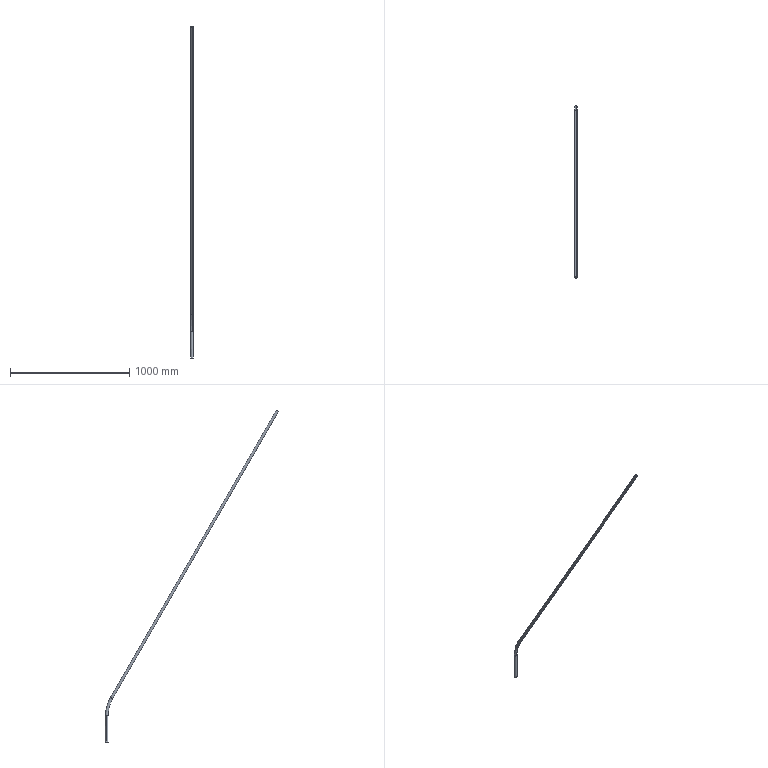Part | SolidWorks | features Sweep 1 | 1 solid | 14 faces | box 22 x 1453 x 2786 mm | volume 397136 mm3 | cylinder 8 | torus 4 | plane 2 | commonest cylinder face diameters 18 x4 22 x4
STEP:
#1=CARTESIAN_POINT('',(-9.,0.,219.615));
#2=VERTEX_POINT('',#1);
#3=CARTESIAN_POINT('',(0.,9.,219.615));
#4=VERTEX_POINT('',#3);
#5=CARTESIAN_POINT('',(0.,0.,219.615));
#6=DIRECTION('',(0.,0.,-1.));
#7=DIRECTION('',(1.,0.,0.));
#8=AXIS2_PLACEMENT_3D('',#5,#6,#7);
#9=CIRCLE('',#8,9.);
#10=EDGE_CURVE('',#2,#4,#9,.T.);
#11=ORIENTED_EDGE('',*,*,#10,.T.);
#12=CARTESIAN_POINT('',(0.,-32.398,374.115));
#13=VERTEX_POINT('',#12);
#14=CARTESIAN_POINT('',(0.,-300.,219.615));
#15=DIRECTION('',(1.,0.,0.));
#16=DIRECTION('',(0.,0.,-1.));
#17=AXIS2_PLACEMENT_3D('',#14,#15,#16);
#18=CIRCLE('',#17,309.);
#19=EDGE_CURVE('',#4,#13,#18,.T.);
#20=ORIENTED_EDGE('',*,*,#19,.T.);
#21=CARTESIAN_POINT('',(0.,-47.987,365.115));
#22=VERTEX_POINT('',#21);
#23=CARTESIAN_POINT('',(0.,-40.192,369.615));
#24=DIRECTION('',(0.,0.5,-0.866));
#25=DIRECTION('',(1.,0.,0.));
#26=AXIS2_PLACEMENT_3D('',#23,#24,#25);
#27=CIRCLE('',#26,9.);
#28=EDGE_CURVE('',#22,#13,#27,.T.);
#29=ORIENTED_EDGE('',*,*,#28,.F.);
#30=CARTESIAN_POINT('',(0.,-9.,219.615));
#31=VERTEX_POINT('',#30);
#32=CARTESIAN_POINT('',(0.,-300.,219.615));
#33=DIRECTION('',(1.,0.,0.));
#34=DIRECTION('',(0.,0.,-1.));
#35=AXIS2_PLACEMENT_3D('',#32,#33,#34);
#36=CIRCLE('',#35,291.);
#37=EDGE_CURVE('',#31,#22,#36,.T.);
#38=ORIENTED_EDGE('',*,*,#37,.F.);
#39=CARTESIAN_POINT('',(0.,0.,219.615));
#40=DIRECTION('',(0.,0.,-1.));
#41=DIRECTION('',(1.,0.,0.));
#42=AXIS2_PLACEMENT_3D('',#39,#40,#41);
#43=CIRCLE('',#42,9.);
#44=EDGE_CURVE('',#31,#2,#43,.T.);
#45=ORIENTED_EDGE('',*,*,#44,.T.);
#46=EDGE_LOOP('',(#11,#20,#29,#38,#45));
#47=FACE_OUTER_BOUND('',#46,.T.);
#48=CARTESIAN_POINT('',(0.,-300.,219.615));
#49=DIRECTION('',(1.,0.,0.));
#50=DIRECTION('',(0.,0.,-1.));
#51=AXIS2_PLACEMENT_3D('',#48,#49,#50);
#52=TOROIDAL_SURFACE('',#51,300.,9.);
#53=ADVANCED_FACE('',(#47),#52,.F.);
#54=CARTESIAN_POINT('',(11.,0.,219.615));
#55=VERTEX_POINT('',#54);
#56=CARTESIAN_POINT('',(0.,11.,219.615));
#57=VERTEX_POINT('',#56);
#58=CARTESIAN_POINT('',(0.,0.,219.615));
#59=DIRECTION('',(0.,0.,1.));
#60=DIRECTION('',(1.,0.,0.));
#61=AXIS2_PLACEMENT_3D('',#58,#59,#60);
#62=CIRCLE('',#61,11.);
#63=EDGE_CURVE('',#55,#57,#62,.T.);
#64=ORIENTED_EDGE('',*,*,#63,.T.);
#65=CARTESIAN_POINT('',(0.,-30.666,375.115));
#66=VERTEX_POINT('',#65);
#67=CARTESIAN_POINT('',(0.,-300.,219.615));
#68=DIRECTION('',(1.,0.,0.));
#69=DIRECTION('',(0.,0.,-1.));
#70=AXIS2_PLACEMENT_3D('',#67,#68,#69);
#71=CIRCLE('',#70,311.);
#72=EDGE_CURVE('',#57,#66,#71,.T.);
#73=ORIENTED_EDGE('',*,*,#72,.T.);
#74=CARTESIAN_POINT('',(0.,-49.719,364.115));
#75=VERTEX_POINT('',#74);
#76=CARTESIAN_POINT('',(0.,-40.192,369.615));
#77=DIRECTION('',(0.,-0.5,0.866));
#78=DIRECTION('',(1.,0.,0.));
#79=AXIS2_PLACEMENT_3D('',#76,#77,#78);
#80=CIRCLE('',#79,11.);
#81=EDGE_CURVE('',#75,#66,#80,.T.);
#82=ORIENTED_EDGE('',*,*,#81,.F.);
#83=CARTESIAN_POINT('',(0.,-11.,219.615));
#84=VERTEX_POINT('',#83);
#85=CARTESIAN_POINT('',(0.,-300.,219.615));
#86=DIRECTION('',(1.,0.,0.));
#87=DIRECTION('',(0.,0.,-1.));
#88=AXIS2_PLACEMENT_3D('',#85,#86,#87);
#89=CIRCLE('',#88,289.);
#90=EDGE_CURVE('',#84,#75,#89,.T.);
#91=ORIENTED_EDGE('',*,*,#90,.F.);
#92=CARTESIAN_POINT('',(0.,0.,219.615));
#93=DIRECTION('',(0.,0.,1.));
#94=DIRECTION('',(1.,0.,0.));
#95=AXIS2_PLACEMENT_3D('',#92,#93,#94);
#96=CIRCLE('',#95,11.);
#97=EDGE_CURVE('',#84,#55,#96,.T.);
#98=ORIENTED_EDGE('',*,*,#97,.T.);
#99=EDGE_LOOP('',(#64,#73,#82,#91,#98));
#100=FACE_OUTER_BOUND('',#99,.T.);
#101=CARTESIAN_POINT('',(0.,-300.,219.615));
#102=DIRECTION('',(1.,0.,0.));
#103=DIRECTION('',(0.,0.,-1.));
#104=AXIS2_PLACEMENT_3D('',#101,#102,#103);
#105=TOROIDAL_SURFACE('',#104,300.,11.);
#106=ADVANCED_FACE('',(#100),#105,.T.);
#107=ORIENTED_EDGE('',*,*,#28,.T.);
#108=CARTESIAN_POINT('',(0.,-1424.206,2784.797));
#109=VERTEX_POINT('',#108);
#110=CARTESIAN_POINT('',(0.,-32.398,374.115));
#111=DIRECTION('',(0.,-0.5,0.866));
#112=VECTOR('',#111,1000.);
#113=LINE('',#110,#112);
#114=EDGE_CURVE('',#13,#109,#113,.T.);
#115=ORIENTED_EDGE('',*,*,#114,.T.);
#116=CARTESIAN_POINT('',(0.,-1439.794,2775.797));
#117=VERTEX_POINT('',#116);
#118=CARTESIAN_POINT('',(0.,-1432.,2780.297));
#119=DIRECTION('',(0.,0.5,-0.866));
#120=DIRECTION('',(1.,0.,0.));
#121=AXIS2_PLACEMENT_3D('',#118,#119,#120);
#122=CIRCLE('',#121,9.);
#123=EDGE_CURVE('',#117,#109,#122,.T.);
#124=ORIENTED_EDGE('',*,*,#123,.F.);
#125=CARTESIAN_POINT('',(0.,-47.987,365.115));
#126=DIRECTION('',(0.,-0.5,0.866));
#127=VECTOR('',#126,1000.);
#128=LINE('',#125,#127);
#129=EDGE_CURVE('',#22,#117,#128,.T.);
#130=ORIENTED_EDGE('',*,*,#129,.F.);
#131=EDGE_LOOP('',(#107,#115,#124,#130));
#132=FACE_OUTER_BOUND('',#131,.T.);
#133=CARTESIAN_POINT('',(0.,-40.192,369.615));
#134=DIRECTION('',(0.,-0.5,0.866));
#135=DIRECTION('',(0.,-0.866,-0.5));
#136=AXIS2_PLACEMENT_3D('',#133,#134,#135);
#137=CYLINDRICAL_SURFACE('',#136,9.);
#138=ADVANCED_FACE('',(#132),#137,.F.);
#139=CARTESIAN_POINT('',(9.,0.,0.));
#140=VERTEX_POINT('',#139);
#141=CARTESIAN_POINT('',(-9.,0.,0.));
#142=VERTEX_POINT('',#141);
#143=CARTESIAN_POINT('',(0.,0.,0.));
#144=DIRECTION('',(0.,0.,-1.));
#145=DIRECTION('',(1.,0.,0.));
#146=AXIS2_PLACEMENT_3D('',#143,#144,#145);
#147=CIRCLE('',#146,9.);
#148=EDGE_CURVE('',#140,#142,#147,.T.);
#149=ORIENTED_EDGE('',*,*,#148,.T.);
#150=CARTESIAN_POINT('',(-9.,0.,0.));
#151=DIRECTION('',(0.,0.,1.));
#152=VECTOR('',#151,1000.);
#153=LINE('',#150,#152);
#154=EDGE_CURVE('',#142,#2,#153,.T.);
#155=ORIENTED_EDGE('',*,*,#154,.T.);
#156=ORIENTED_EDGE('',*,*,#44,.F.);
#157=CARTESIAN_POINT('',(9.,0.,219.615));
#158=VERTEX_POINT('',#157);
#159=CARTESIAN_POINT('',(0.,0.,219.615));
#160=DIRECTION('',(0.,0.,-1.));
#161=DIRECTION('',(1.,0.,0.));
#162=AXIS2_PLACEMENT_3D('',#159,#160,#161);
#163=CIRCLE('',#162,9.);
#164=EDGE_CURVE('',#158,#31,#163,.T.);
#165=ORIENTED_EDGE('',*,*,#164,.F.);
#166=CARTESIAN_POINT('',(9.,0.,0.));
#167=DIRECTION('',(0.,0.,1.));
#168=VECTOR('',#167,1000.);
#169=LINE('',#166,#168);
#170=EDGE_CURVE('',#140,#158,#169,.T.);
#171=ORIENTED_EDGE('',*,*,#170,.F.);
#172=EDGE_LOOP('',(#149,#155,#156,#165,#171));
#173=FACE_OUTER_BOUND('',#172,.T.);
#174=CARTESIAN_POINT('',(0.,0.,0.));
#175=DIRECTION('',(0.,0.,1.));
#176=DIRECTION('',(1.,0.,0.));
#177=AXIS2_PLACEMENT_3D('',#174,#175,#176);
#178=CYLINDRICAL_SURFACE('',#177,9.);
#179=ADVANCED_FACE('',(#173),#178,.F.);
#180=ORIENTED_EDGE('',*,*,#81,.T.);
#181=CARTESIAN_POINT('',(0.,-1422.474,2785.797));
#182=VERTEX_POINT('',#181);
#183=CARTESIAN_POINT('',(0.,-30.666,375.115));
#184=DIRECTION('',(0.,-0.5,0.866));
#185=VECTOR('',#184,1000.);
#186=LINE('',#183,#185);
#187=EDGE_CURVE('',#66,#182,#186,.T.);
#188=ORIENTED_EDGE('',*,*,#187,.T.);
#189=CARTESIAN_POINT('',(0.,-1441.526,2774.797));
#190=VERTEX_POINT('',#189);
#191=CARTESIAN_POINT('',(0.,-1432.,2780.297));
#192=DIRECTION('',(0.,-0.5,0.866));
#193=DIRECTION('',(1.,0.,0.));
#194=AXIS2_PLACEMENT_3D('',#191,#192,#193);
#195=CIRCLE('',#194,11.);
#196=EDGE_CURVE('',#190,#182,#195,.T.);
#197=ORIENTED_EDGE('',*,*,#196,.F.);
#198=CARTESIAN_POINT('',(0.,-49.719,364.115));
#199=DIRECTION('',(0.,-0.5,0.866));
#200=VECTOR('',#199,1000.);
#201=LINE('',#198,#200);
#202=EDGE_CURVE('',#75,#190,#201,.T.);
#203=ORIENTED_EDGE('',*,*,#202,.F.);
#204=EDGE_LOOP('',(#180,#188,#197,#203));
#205=FACE_OUTER_BOUND('',#204,.T.);
#206=CARTESIAN_POINT('',(0.,-40.192,369.615));
#207=DIRECTION('',(0.,-0.5,0.866));
#208=DIRECTION('',(0.,-0.866,-0.5));
#209=AXIS2_PLACEMENT_3D('',#206,#207,#208);
#210=CYLINDRICAL_SURFACE('',#209,11.);
#211=ADVANCED_FACE('',(#205),#210,.T.);
#212=CARTESIAN_POINT('',(11.,0.,0.));
#213=VERTEX_POINT('',#212);
#214=CARTESIAN_POINT('',(-11.,0.,0.));
#215=VERTEX_POINT('',#214);
#216=CARTESIAN_POINT('',(0.,0.,0.));
#217=DIRECTION('',(0.,0.,1.));
#218=DIRECTION('',(1.,0.,0.));
#219=AXIS2_PLACEMENT_3D('',#216,#217,#218);
#220=CIRCLE('',#219,11.);
#221=EDGE_CURVE('',#213,#215,#220,.T.);
#222=ORIENTED_EDGE('',*,*,#221,.T.);
#223=CARTESIAN_POINT('',(-11.,0.,219.615));
#224=VERTEX_POINT('',#223);
#225=CARTESIAN_POINT('',(-11.,0.,0.));
#226=DIRECTION('',(0.,0.,1.));
#227=VECTOR('',#226,1000.);
#228=LINE('',#225,#227);
#229=EDGE_CURVE('',#215,#224,#228,.T.);
#230=ORIENTED_EDGE('',*,*,#229,.T.);
#231=CARTESIAN_POINT('',(0.,0.,219.615));
#232=DIRECTION('',(0.,0.,1.));
#233=DIRECTION('',(1.,0.,0.));
#234=AXIS2_PLACEMENT_3D('',#231,#232,#233);
#235=CIRCLE('',#234,11.);
#236=EDGE_CURVE('',#57,#224,#235,.T.);
#237=ORIENTED_EDGE('',*,*,#236,.F.);
#238=ORIENTED_EDGE('',*,*,#63,.F.);
#239=CARTESIAN_POINT('',(11.,0.,0.));
#240=DIRECTION('',(0.,0.,1.));
#241=VECTOR('',#240,1000.);
#242=LINE('',#239,#241);
#243=EDGE_CURVE('',#213,#55,#242,.T.);
#244=ORIENTED_EDGE('',*,*,#243,.F.);
#245=EDGE_LOOP('',(#222,#230,#237,#238,#244));
#246=FACE_OUTER_BOUND('',#245,.T.);
#247=CARTESIAN_POINT('',(0.,0.,0.));
#248=DIRECTION('',(0.,0.,1.));
#249=DIRECTION('',(1.,0.,0.));
#250=AXIS2_PLACEMENT_3D('',#247,#248,#249);
#251=CYLINDRICAL_SURFACE('',#250,11.);
#252=ADVANCED_FACE('',(#246),#251,.T.);
#253=ORIENTED_EDGE('',*,*,#114,.F.);
#254=CARTESIAN_POINT('',(0.,-40.192,369.615));
#255=DIRECTION('',(0.,0.5,-0.866));
#256=DIRECTION('',(1.,0.,0.));
#257=AXIS2_PLACEMENT_3D('',#254,#255,#256);
#258=CIRCLE('',#257,9.);
#259=EDGE_CURVE('',#13,#22,#258,.T.);
#260=ORIENTED_EDGE('',*,*,#259,.T.);
#261=ORIENTED_EDGE('',*,*,#129,.T.);
#262=CARTESIAN_POINT('',(0.,-1432.,2780.297));
#263=DIRECTION('',(0.,0.5,-0.866));
#264=DIRECTION('',(1.,0.,0.));
#265=AXIS2_PLACEMENT_3D('',#262,#263,#264);
#266=CIRCLE('',#265,9.);
#267=EDGE_CURVE('',#109,#117,#266,.T.);
#268=ORIENTED_EDGE('',*,*,#267,.F.);
#269=EDGE_LOOP('',(#253,#260,#261,#268));
#270=FACE_OUTER_BOUND('',#269,.T.);
#271=CARTESIAN_POINT('',(0.,-40.192,369.615));
#272=DIRECTION('',(0.,-0.5,0.866));
#273=DIRECTION('',(0.,-0.866,-0.5));
#274=AXIS2_PLACEMENT_3D('',#271,#272,#273);
#275=CYLINDRICAL_SURFACE('',#274,9.);
#276=ADVANCED_FACE('',(#270),#275,.F.);
#277=ORIENTED_EDGE('',*,*,#19,.F.);
#278=CARTESIAN_POINT('',(0.,0.,219.615));
#279=DIRECTION('',(0.,0.,-1.));
#280=DIRECTION('',(1.,0.,0.));
#281=AXIS2_PLACEMENT_3D('',#278,#279,#280);
#282=CIRCLE('',#281,9.);
#283=EDGE_CURVE('',#4,#158,#282,.T.);
#284=ORIENTED_EDGE('',*,*,#283,.T.);
#285=ORIENTED_EDGE('',*,*,#164,.T.);
#286=ORIENTED_EDGE('',*,*,#37,.T.);
#287=ORIENTED_EDGE('',*,*,#259,.F.);
#288=EDGE_LOOP('',(#277,#284,#285,#286,#287));
#289=FACE_OUTER_BOUND('',#288,.T.);
#290=CARTESIAN_POINT('',(0.,-300.,219.615));
#291=DIRECTION('',(1.,0.,0.));
#292=DIRECTION('',(0.,0.,-1.));
#293=AXIS2_PLACEMENT_3D('',#290,#291,#292);
#294=TOROIDAL_SURFACE('',#293,300.,9.);
#295=ADVANCED_FACE('',(#289),#294,.F.);
#296=ORIENTED_EDGE('',*,*,#154,.F.);
#297=CARTESIAN_POINT('',(0.,0.,0.));
#298=DIRECTION('',(0.,0.,-1.));
#299=DIRECTION('',(1.,0.,0.));
#300=AXIS2_PLACEMENT_3D('',#297,#298,#299);
#301=CIRCLE('',#300,9.);
#302=EDGE_CURVE('',#142,#140,#301,.T.);
#303=ORIENTED_EDGE('',*,*,#302,.T.);
#304=ORIENTED_EDGE('',*,*,#170,.T.);
#305=ORIENTED_EDGE('',*,*,#283,.F.);
#306=ORIENTED_EDGE('',*,*,#10,.F.);
#307=EDGE_LOOP('',(#296,#303,#304,#305,#306));
#308=FACE_OUTER_BOUND('',#307,.T.);
#309=CARTESIAN_POINT('',(0.,0.,0.));
#310=DIRECTION('',(0.,0.,1.));
#311=DIRECTION('',(1.,0.,0.));
#312=AXIS2_PLACEMENT_3D('',#309,#310,#311);
#313=CYLINDRICAL_SURFACE('',#312,9.);
#314=ADVANCED_FACE('',(#308),#313,.F.);
#315=ORIENTED_EDGE('',*,*,#123,.T.);
#316=ORIENTED_EDGE('',*,*,#267,.T.);
#317=EDGE_LOOP('',(#315,#316));
#318=FACE_BOUND('',#317,.T.);
#319=ORIENTED_EDGE('',*,*,#196,.T.);
#320=CARTESIAN_POINT('',(0.,-1432.,2780.297));
#321=DIRECTION('',(0.,-0.5,0.866));
#322=DIRECTION('',(1.,0.,0.));
#323=AXIS2_PLACEMENT_3D('',#320,#321,#322);
#324=CIRCLE('',#323,11.);
#325=EDGE_CURVE('',#182,#190,#324,.T.);
#326=ORIENTED_EDGE('',*,*,#325,.T.);
#327=EDGE_LOOP('',(#319,#326));
#328=FACE_OUTER_BOUND('',#327,.T.);
#329=CARTESIAN_POINT('',(0.,-1432.,2780.297));
#330=DIRECTION('',(0.,-0.5,0.866));
#331=DIRECTION('',(1.,0.,0.));
#332=AXIS2_PLACEMENT_3D('',#329,#330,#331);
#333=PLANE('',#332);
#334=ADVANCED_FACE('',(#318,#328),#333,.T.);
#335=ORIENTED_EDGE('',*,*,#148,.F.);
#336=ORIENTED_EDGE('',*,*,#302,.F.);
#337=EDGE_LOOP('',(#335,#336));
#338=FACE_BOUND('',#337,.T.);
#339=ORIENTED_EDGE('',*,*,#221,.F.);
#340=CARTESIAN_POINT('',(0.,0.,0.));
#341=DIRECTION('',(0.,0.,1.));
#342=DIRECTION('',(1.,0.,0.));
#343=AXIS2_PLACEMENT_3D('',#340,#341,#342);
#344=CIRCLE('',#343,11.);
#345=EDGE_CURVE('',#215,#213,#344,.T.);
#346=ORIENTED_EDGE('',*,*,#345,.F.);
#347=EDGE_LOOP('',(#339,#346));
#348=FACE_OUTER_BOUND('',#347,.T.);
#349=CARTESIAN_POINT('',(0.,0.,0.));
#350=DIRECTION('',(0.,0.,1.));
#351=DIRECTION('',(1.,0.,0.));
#352=AXIS2_PLACEMENT_3D('',#349,#350,#351);
#353=PLANE('',#352);
#354=ADVANCED_FACE('',(#338,#348),#353,.F.);
#355=ORIENTED_EDGE('',*,*,#187,.F.);
#356=CARTESIAN_POINT('',(0.,-40.192,369.615));
#357=DIRECTION('',(0.,-0.5,0.866));
#358=DIRECTION('',(1.,0.,0.));
#359=AXIS2_PLACEMENT_3D('',#356,#357,#358);
#360=CIRCLE('',#359,11.);
#361=EDGE_CURVE('',#66,#75,#360,.T.);
#362=ORIENTED_EDGE('',*,*,#361,.T.);
#363=ORIENTED_EDGE('',*,*,#202,.T.);
#364=ORIENTED_EDGE('',*,*,#325,.F.);
#365=EDGE_LOOP('',(#355,#362,#363,#364));
#366=FACE_OUTER_BOUND('',#365,.T.);
#367=CARTESIAN_POINT('',(0.,-40.192,369.615));
#368=DIRECTION('',(0.,-0.5,0.866));
#369=DIRECTION('',(0.,-0.866,-0.5));
#370=AXIS2_PLACEMENT_3D('',#367,#368,#369);
#371=CYLINDRICAL_SURFACE('',#370,11.);
#372=ADVANCED_FACE('',(#366),#371,.T.);
#373=ORIENTED_EDGE('',*,*,#72,.F.);
#374=ORIENTED_EDGE('',*,*,#236,.T.);
#375=CARTESIAN_POINT('',(0.,0.,219.615));
#376=DIRECTION('',(0.,0.,1.));
#377=DIRECTION('',(1.,0.,0.));
#378=AXIS2_PLACEMENT_3D('',#375,#376,#377);
#379=CIRCLE('',#378,11.);
#380=EDGE_CURVE('',#224,#84,#379,.T.);
#381=ORIENTED_EDGE('',*,*,#380,.T.);
#382=ORIENTED_EDGE('',*,*,#90,.T.);
#383=ORIENTED_EDGE('',*,*,#361,.F.);
#384=EDGE_LOOP('',(#373,#374,#381,#382,#383));
#385=FACE_OUTER_BOUND('',#384,.T.);
#386=CARTESIAN_POINT('',(0.,-300.,219.615));
#387=DIRECTION('',(1.,0.,0.));
#388=DIRECTION('',(0.,0.,-1.));
#389=AXIS2_PLACEMENT_3D('',#386,#387,#388);
#390=TOROIDAL_SURFACE('',#389,300.,11.);
#391=ADVANCED_FACE('',(#385),#390,.T.);
#392=ORIENTED_EDGE('',*,*,#229,.F.);
#393=ORIENTED_EDGE('',*,*,#345,.T.);
#394=ORIENTED_EDGE('',*,*,#243,.T.);
#395=ORIENTED_EDGE('',*,*,#97,.F.);
#396=ORIENTED_EDGE('',*,*,#380,.F.);
#397=EDGE_LOOP('',(#392,#393,#394,#395,#396));
#398=FACE_OUTER_BOUND('',#397,.T.);
#399=CARTESIAN_POINT('',(0.,0.,0.));
#400=DIRECTION('',(0.,0.,1.));
#401=DIRECTION('',(1.,0.,0.));
#402=AXIS2_PLACEMENT_3D('',#399,#400,#401);
#403=CYLINDRICAL_SURFACE('',#402,11.);
#404=ADVANCED_FACE('',(#398),#403,.T.);
#405=CLOSED_SHELL('',(#53,#106,#138,#179,#211,#252,#276,#295,#314,#334,#354,#372,#391,#404));
#406=MANIFOLD_SOLID_BREP('',#405);
#407=CARTESIAN_POINT('',(0.,0.,0.));
#408=DIRECTION('',(0.,0.,1.));
#409=DIRECTION('',(1.,0.,0.));
#410=AXIS2_PLACEMENT_3D('',#407,#408,#409);
#411=(LENGTH_UNIT()NAMED_UNIT(*)SI_UNIT(.MILLI.,.METRE.));
#412=UNCERTAINTY_MEASURE_WITH_UNIT(LENGTH_MEASURE(0.00001),#411,'','');
#413=(NAMED_UNIT(*)PLANE_ANGLE_UNIT()SI_UNIT($,.RADIAN.));
#414=(NAMED_UNIT(*)SI_UNIT($,.STERADIAN.)SOLID_ANGLE_UNIT());
#415=(GEOMETRIC_REPRESENTATION_CONTEXT(3)GLOBAL_UNCERTAINTY_ASSIGNED_CONTEXT((#412))GLOBAL_UNIT_ASSIGNED_CONTEXT((#411,#413,#414))REPRESENTATION_CONTEXT('',''));
#416=ADVANCED_BREP_SHAPE_REPRESENTATION('',(#406,#410),#415);